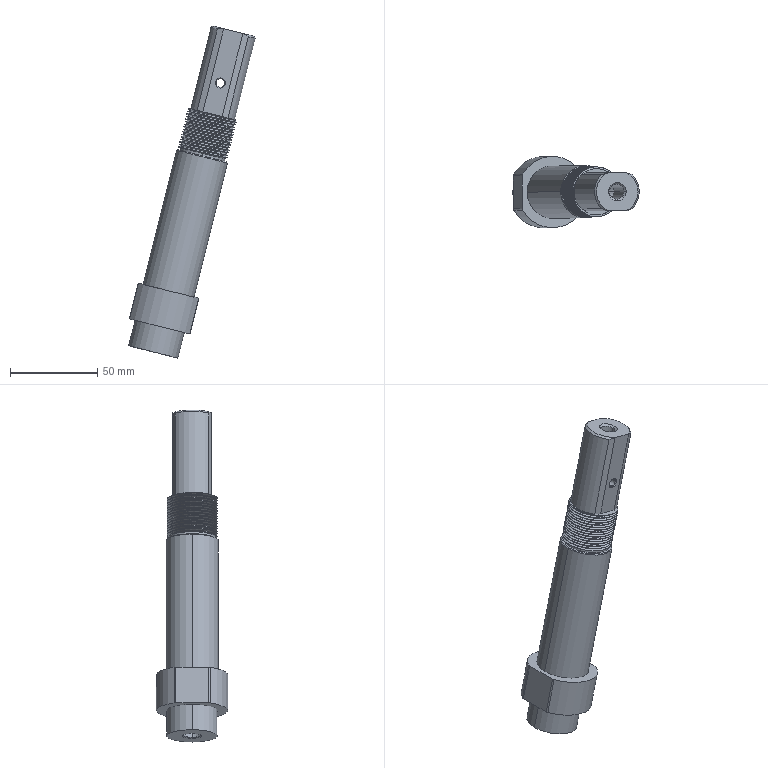Part | SolidWorks | features BaseBody 1 | 1 solid | 119 faces | box 72.376 x 40.8 x 189.852 mm | volume 126579 mm3 | cylinder 84 | plane 16 | cone 15 | spline 4 | commonest cylinder face diameters 26.5 x33 28.6 x32 4 x4 40.8 x3 4.8 x2 8.5 x2